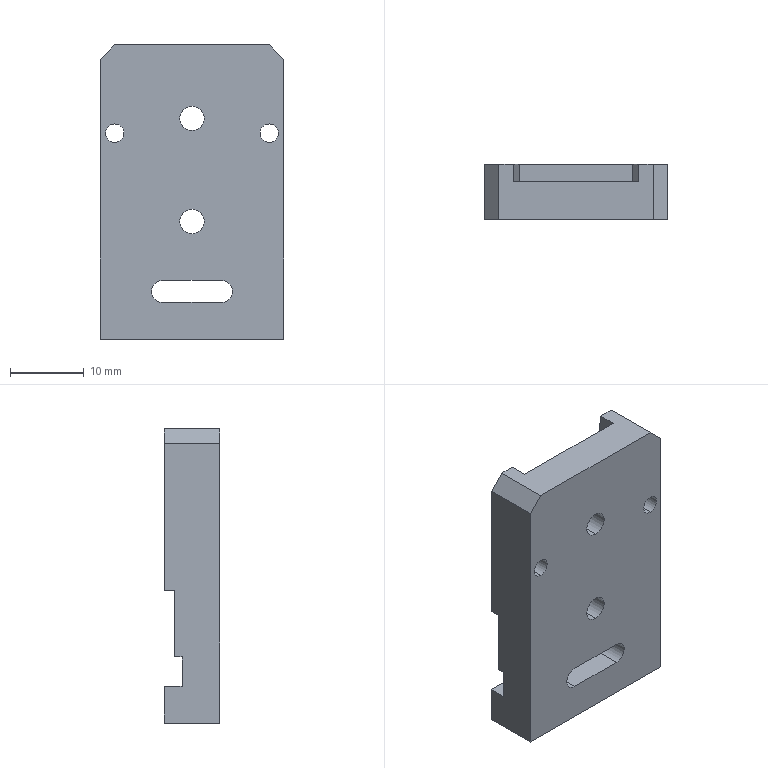Part | STEP file | PN_0042 Mount electronic clip fixed groove | 1 solid | 33 faces | box 25 x 7.5 x 40 mm | volume 5632 mm3 | plane 23 | cylinder 10 | commonest cylinder face diameters 2.5 x4 3.3 x4 3 x2